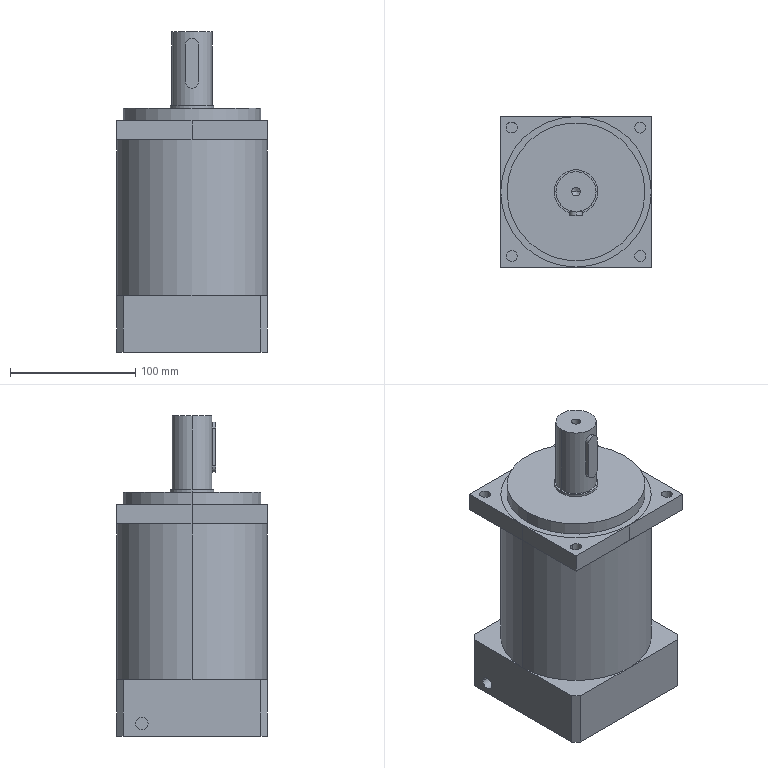Part | SolidWorks | features Boss 5, ICE 3, CirPattern 2, HoleWzd 2, Chamfer 1, Cut 1, Extrusion 1 | 6 solids | 86 faces | box 120 x 120 x 255.5 mm | volume 2340671 mm3 | plane 39 | cylinder 37 | cone 10 | commonest cylinder face diameters 6.8 x8 8.8 x8 120 x6 10 x5 110 x4 7 x2